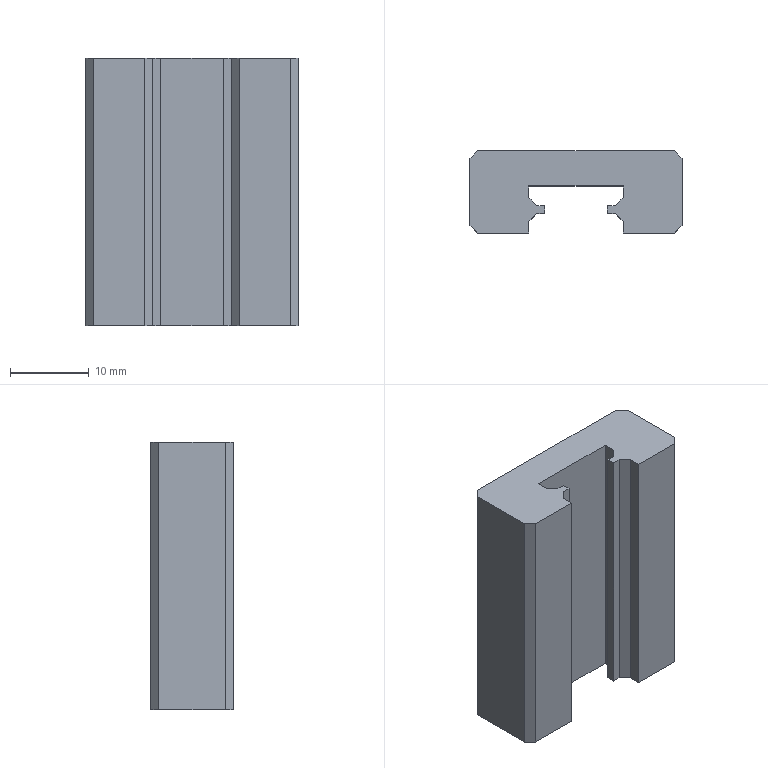Part | SolidWorks | features Chamfer 1, Extrusion 1 | 1 solid | 26 faces | box 27 x 10.5 x 34 mm | volume 7327 mm3 | plane 26
STEP:
#1=CARTESIAN_POINT('',(6.,-5.5,0.));
#2=VERTEX_POINT('',#1);
#3=CARTESIAN_POINT('',(12.5,-5.5,0.));
#4=VERTEX_POINT('',#3);
#5=CARTESIAN_POINT('',(6.,-5.5,0.));
#6=DIRECTION('',(1.,0.,0.));
#7=VECTOR('',#6,1000.);
#8=LINE('',#5,#7);
#9=EDGE_CURVE('',#2,#4,#8,.T.);
#10=ORIENTED_EDGE('',*,*,#9,.T.);
#11=CARTESIAN_POINT('',(12.5,-5.5,34.));
#12=VERTEX_POINT('',#11);
#13=CARTESIAN_POINT('',(12.5,-5.5,34.));
#14=DIRECTION('',(0.,0.,1.));
#15=VECTOR('',#14,1000.);
#16=LINE('',#13,#15);
#17=EDGE_CURVE('',#4,#12,#16,.T.);
#18=ORIENTED_EDGE('',*,*,#17,.T.);
#19=CARTESIAN_POINT('',(6.,-5.5,34.));
#20=VERTEX_POINT('',#19);
#21=CARTESIAN_POINT('',(6.,-5.5,34.));
#22=DIRECTION('',(1.,0.,0.));
#23=VECTOR('',#22,1000.);
#24=LINE('',#21,#23);
#25=EDGE_CURVE('',#20,#12,#24,.T.);
#26=ORIENTED_EDGE('',*,*,#25,.F.);
#27=CARTESIAN_POINT('',(6.,-5.5,34.));
#28=DIRECTION('',(0.,0.,-1.));
#29=VECTOR('',#28,1000.);
#30=LINE('',#27,#29);
#31=EDGE_CURVE('',#20,#2,#30,.T.);
#32=ORIENTED_EDGE('',*,*,#31,.T.);
#33=EDGE_LOOP('',(#10,#18,#26,#32));
#34=FACE_OUTER_BOUND('',#33,.T.);
#35=CARTESIAN_POINT('',(6.,-5.5,34.));
#36=DIRECTION('',(0.,1.,0.));
#37=DIRECTION('',(0.,0.,1.));
#38=AXIS2_PLACEMENT_3D('',#35,#36,#37);
#39=PLANE('',#38);
#40=ADVANCED_FACE('',(#34),#39,.F.);
#41=CARTESIAN_POINT('',(13.5,-4.5,34.));
#42=VERTEX_POINT('',#41);
#43=CARTESIAN_POINT('',(13.5,4.,34.));
#44=VERTEX_POINT('',#43);
#45=CARTESIAN_POINT('',(13.5,5.,34.));
#46=DIRECTION('',(0.,1.,0.));
#47=VECTOR('',#46,1000.);
#48=LINE('',#45,#47);
#49=EDGE_CURVE('',#42,#44,#48,.T.);
#50=ORIENTED_EDGE('',*,*,#49,.F.);
#51=CARTESIAN_POINT('',(13.5,-4.5,0.));
#52=VERTEX_POINT('',#51);
#53=CARTESIAN_POINT('',(13.5,-4.5,34.));
#54=DIRECTION('',(0.,0.,-1.));
#55=VECTOR('',#54,1000.);
#56=LINE('',#53,#55);
#57=EDGE_CURVE('',#42,#52,#56,.T.);
#58=ORIENTED_EDGE('',*,*,#57,.T.);
#59=CARTESIAN_POINT('',(13.5,4.,0.));
#60=VERTEX_POINT('',#59);
#61=CARTESIAN_POINT('',(13.5,5.,0.));
#62=DIRECTION('',(0.,1.,0.));
#63=VECTOR('',#62,1000.);
#64=LINE('',#61,#63);
#65=EDGE_CURVE('',#52,#60,#64,.T.);
#66=ORIENTED_EDGE('',*,*,#65,.T.);
#67=CARTESIAN_POINT('',(13.5,4.,34.));
#68=DIRECTION('',(0.,0.,1.));
#69=VECTOR('',#68,1000.);
#70=LINE('',#67,#69);
#71=EDGE_CURVE('',#60,#44,#70,.T.);
#72=ORIENTED_EDGE('',*,*,#71,.T.);
#73=EDGE_LOOP('',(#50,#58,#66,#72));
#74=FACE_OUTER_BOUND('',#73,.T.);
#75=CARTESIAN_POINT('',(13.5,5.,34.));
#76=DIRECTION('',(-1.,0.,0.));
#77=DIRECTION('',(0.,-1.,0.));
#78=AXIS2_PLACEMENT_3D('',#75,#76,#77);
#79=PLANE('',#78);
#80=ADVANCED_FACE('',(#74),#79,.F.);
#81=CARTESIAN_POINT('',(12.5,5.,0.));
#82=VERTEX_POINT('',#81);
#83=CARTESIAN_POINT('',(-12.5,5.,0.));
#84=VERTEX_POINT('',#83);
#85=CARTESIAN_POINT('',(-13.5,5.,0.));
#86=DIRECTION('',(-1.,0.,0.));
#87=VECTOR('',#86,1000.);
#88=LINE('',#85,#87);
#89=EDGE_CURVE('',#82,#84,#88,.T.);
#90=ORIENTED_EDGE('',*,*,#89,.T.);
#91=CARTESIAN_POINT('',(-12.5,5.,34.));
#92=VERTEX_POINT('',#91);
#93=CARTESIAN_POINT('',(-12.5,5.,34.));
#94=DIRECTION('',(0.,0.,1.));
#95=VECTOR('',#94,1000.);
#96=LINE('',#93,#95);
#97=EDGE_CURVE('',#84,#92,#96,.T.);
#98=ORIENTED_EDGE('',*,*,#97,.T.);
#99=CARTESIAN_POINT('',(12.5,5.,34.));
#100=VERTEX_POINT('',#99);
#101=CARTESIAN_POINT('',(-13.5,5.,34.));
#102=DIRECTION('',(-1.,0.,0.));
#103=VECTOR('',#102,1000.);
#104=LINE('',#101,#103);
#105=EDGE_CURVE('',#100,#92,#104,.T.);
#106=ORIENTED_EDGE('',*,*,#105,.F.);
#107=CARTESIAN_POINT('',(12.5,5.,34.));
#108=DIRECTION('',(0.,0.,-1.));
#109=VECTOR('',#108,1000.);
#110=LINE('',#107,#109);
#111=EDGE_CURVE('',#100,#82,#110,.T.);
#112=ORIENTED_EDGE('',*,*,#111,.T.);
#113=EDGE_LOOP('',(#90,#98,#106,#112));
#114=FACE_OUTER_BOUND('',#113,.T.);
#115=CARTESIAN_POINT('',(-13.5,5.,34.));
#116=DIRECTION('',(0.,-1.,0.));
#117=DIRECTION('',(0.,0.,-1.));
#118=AXIS2_PLACEMENT_3D('',#115,#116,#117);
#119=PLANE('',#118);
#120=ADVANCED_FACE('',(#114),#119,.F.);
#121=CARTESIAN_POINT('',(-13.5,4.,0.));
#122=VERTEX_POINT('',#121);
#123=CARTESIAN_POINT('',(-13.5,-4.5,0.));
#124=VERTEX_POINT('',#123);
#125=CARTESIAN_POINT('',(-13.5,5.,0.));
#126=DIRECTION('',(0.,-1.,0.));
#127=VECTOR('',#126,1000.);
#128=LINE('',#125,#127);
#129=EDGE_CURVE('',#122,#124,#128,.T.);
#130=ORIENTED_EDGE('',*,*,#129,.T.);
#131=CARTESIAN_POINT('',(-13.5,-4.5,34.));
#132=VERTEX_POINT('',#131);
#133=CARTESIAN_POINT('',(-13.5,-4.5,34.));
#134=DIRECTION('',(0.,0.,1.));
#135=VECTOR('',#134,1000.);
#136=LINE('',#133,#135);
#137=EDGE_CURVE('',#124,#132,#136,.T.);
#138=ORIENTED_EDGE('',*,*,#137,.T.);
#139=CARTESIAN_POINT('',(-13.5,4.,34.));
#140=VERTEX_POINT('',#139);
#141=CARTESIAN_POINT('',(-13.5,5.,34.));
#142=DIRECTION('',(0.,-1.,0.));
#143=VECTOR('',#142,1000.);
#144=LINE('',#141,#143);
#145=EDGE_CURVE('',#140,#132,#144,.T.);
#146=ORIENTED_EDGE('',*,*,#145,.F.);
#147=CARTESIAN_POINT('',(-13.5,4.,34.));
#148=DIRECTION('',(0.,0.,-1.));
#149=VECTOR('',#148,1000.);
#150=LINE('',#147,#149);
#151=EDGE_CURVE('',#140,#122,#150,.T.);
#152=ORIENTED_EDGE('',*,*,#151,.T.);
#153=EDGE_LOOP('',(#130,#138,#146,#152));
#154=FACE_OUTER_BOUND('',#153,.T.);
#155=CARTESIAN_POINT('',(-13.5,5.,34.));
#156=DIRECTION('',(1.,0.,0.));
#157=DIRECTION('',(0.,1.,0.));
#158=AXIS2_PLACEMENT_3D('',#155,#156,#157);
#159=PLANE('',#158);
#160=ADVANCED_FACE('',(#154),#159,.F.);
#161=CARTESIAN_POINT('',(-12.5,-5.5,34.));
#162=VERTEX_POINT('',#161);
#163=CARTESIAN_POINT('',(-6.,-5.5,34.));
#164=VERTEX_POINT('',#163);
#165=CARTESIAN_POINT('',(-13.5,-5.5,34.));
#166=DIRECTION('',(1.,0.,0.));
#167=VECTOR('',#166,1000.);
#168=LINE('',#165,#167);
#169=EDGE_CURVE('',#162,#164,#168,.T.);
#170=ORIENTED_EDGE('',*,*,#169,.F.);
#171=CARTESIAN_POINT('',(-12.5,-5.5,0.));
#172=VERTEX_POINT('',#171);
#173=CARTESIAN_POINT('',(-12.5,-5.5,34.));
#174=DIRECTION('',(0.,0.,-1.));
#175=VECTOR('',#174,1000.);
#176=LINE('',#173,#175);
#177=EDGE_CURVE('',#162,#172,#176,.T.);
#178=ORIENTED_EDGE('',*,*,#177,.T.);
#179=CARTESIAN_POINT('',(-6.,-5.5,0.));
#180=VERTEX_POINT('',#179);
#181=CARTESIAN_POINT('',(-13.5,-5.5,0.));
#182=DIRECTION('',(1.,0.,0.));
#183=VECTOR('',#182,1000.);
#184=LINE('',#181,#183);
#185=EDGE_CURVE('',#172,#180,#184,.T.);
#186=ORIENTED_EDGE('',*,*,#185,.T.);
#187=CARTESIAN_POINT('',(-6.,-5.5,34.));
#188=DIRECTION('',(0.,0.,-1.));
#189=VECTOR('',#188,1000.);
#190=LINE('',#187,#189);
#191=EDGE_CURVE('',#164,#180,#190,.T.);
#192=ORIENTED_EDGE('',*,*,#191,.F.);
#193=EDGE_LOOP('',(#170,#178,#186,#192));
#194=FACE_OUTER_BOUND('',#193,.T.);
#195=CARTESIAN_POINT('',(-13.5,-5.5,34.));
#196=DIRECTION('',(0.,1.,0.));
#197=DIRECTION('',(0.,0.,1.));
#198=AXIS2_PLACEMENT_3D('',#195,#196,#197);
#199=PLANE('',#198);
#200=ADVANCED_FACE('',(#194),#199,.F.);
#201=CARTESIAN_POINT('',(-6.,-4.,0.));
#202=VERTEX_POINT('',#201);
#203=CARTESIAN_POINT('',(-6.,-4.,0.));
#204=DIRECTION('',(0.,1.,0.));
#205=VECTOR('',#204,1000.);
#206=LINE('',#203,#205);
#207=EDGE_CURVE('',#180,#202,#206,.T.);
#208=ORIENTED_EDGE('',*,*,#207,.T.);
#209=CARTESIAN_POINT('',(-6.,-4.,34.));
#210=VERTEX_POINT('',#209);
#211=CARTESIAN_POINT('',(-6.,-4.,34.));
#212=DIRECTION('',(0.,0.,-1.));
#213=VECTOR('',#212,1000.);
#214=LINE('',#211,#213);
#215=EDGE_CURVE('',#210,#202,#214,.T.);
#216=ORIENTED_EDGE('',*,*,#215,.F.);
#217=CARTESIAN_POINT('',(-6.,-4.,34.));
#218=DIRECTION('',(0.,1.,0.));
#219=VECTOR('',#218,1000.);
#220=LINE('',#217,#219);
#221=EDGE_CURVE('',#164,#210,#220,.T.);
#222=ORIENTED_EDGE('',*,*,#221,.F.);
#223=ORIENTED_EDGE('',*,*,#191,.T.);
#224=EDGE_LOOP('',(#208,#216,#222,#223));
#225=FACE_OUTER_BOUND('',#224,.T.);
#226=CARTESIAN_POINT('',(-6.,-4.,34.));
#227=DIRECTION('',(-1.,0.,0.));
#228=DIRECTION('',(0.,-1.,0.));
#229=AXIS2_PLACEMENT_3D('',#226,#227,#228);
#230=PLANE('',#229);
#231=ADVANCED_FACE('',(#225),#230,.F.);
#232=CARTESIAN_POINT('',(-5.,-3.,0.));
#233=VERTEX_POINT('',#232);
#234=CARTESIAN_POINT('',(-5.,-3.,0.));
#235=DIRECTION('',(0.7071,0.7071,0.));
#236=VECTOR('',#235,1000.);
#237=LINE('',#234,#236);
#238=EDGE_CURVE('',#202,#233,#237,.T.);
#239=ORIENTED_EDGE('',*,*,#238,.T.);
#240=CARTESIAN_POINT('',(-5.,-3.,34.));
#241=VERTEX_POINT('',#240);
#242=CARTESIAN_POINT('',(-5.,-3.,34.));
#243=DIRECTION('',(0.,0.,-1.));
#244=VECTOR('',#243,1000.);
#245=LINE('',#242,#244);
#246=EDGE_CURVE('',#241,#233,#245,.T.);
#247=ORIENTED_EDGE('',*,*,#246,.F.);
#248=CARTESIAN_POINT('',(-5.,-3.,34.));
#249=DIRECTION('',(0.7071,0.7071,0.));
#250=VECTOR('',#249,1000.);
#251=LINE('',#248,#250);
#252=EDGE_CURVE('',#210,#241,#251,.T.);
#253=ORIENTED_EDGE('',*,*,#252,.F.);
#254=ORIENTED_EDGE('',*,*,#215,.T.);
#255=EDGE_LOOP('',(#239,#247,#253,#254));
#256=FACE_OUTER_BOUND('',#255,.T.);
#257=CARTESIAN_POINT('',(-5.,-3.,34.));
#258=DIRECTION('',(-0.7071,0.7071,0.));
#259=DIRECTION('',(-0.7071,-0.7071,0.));
#260=AXIS2_PLACEMENT_3D('',#257,#258,#259);
#261=PLANE('',#260);
#262=ADVANCED_FACE('',(#256),#261,.F.);
#263=CARTESIAN_POINT('',(-4.,-3.,0.));
#264=VERTEX_POINT('',#263);
#265=CARTESIAN_POINT('',(-4.,-3.,0.));
#266=DIRECTION('',(1.,0.,0.));
#267=VECTOR('',#266,1000.);
#268=LINE('',#265,#267);
#269=EDGE_CURVE('',#233,#264,#268,.T.);
#270=ORIENTED_EDGE('',*,*,#269,.T.);
#271=CARTESIAN_POINT('',(-4.,-3.,34.));
#272=VERTEX_POINT('',#271);
#273=CARTESIAN_POINT('',(-4.,-3.,34.));
#274=DIRECTION('',(0.,0.,-1.));
#275=VECTOR('',#274,1000.);
#276=LINE('',#273,#275);
#277=EDGE_CURVE('',#272,#264,#276,.T.);
#278=ORIENTED_EDGE('',*,*,#277,.F.);
#279=CARTESIAN_POINT('',(-4.,-3.,34.));
#280=DIRECTION('',(1.,0.,0.));
#281=VECTOR('',#280,1000.);
#282=LINE('',#279,#281);
#283=EDGE_CURVE('',#241,#272,#282,.T.);
#284=ORIENTED_EDGE('',*,*,#283,.F.);
#285=ORIENTED_EDGE('',*,*,#246,.T.);
#286=EDGE_LOOP('',(#270,#278,#284,#285));
#287=FACE_OUTER_BOUND('',#286,.T.);
#288=CARTESIAN_POINT('',(-4.,-3.,34.));
#289=DIRECTION('',(0.,1.,0.));
#290=DIRECTION('',(0.,0.,1.));
#291=AXIS2_PLACEMENT_3D('',#288,#289,#290);
#292=PLANE('',#291);
#293=ADVANCED_FACE('',(#287),#292,.F.);
#294=CARTESIAN_POINT('',(-4.,-2.,0.));
#295=VERTEX_POINT('',#294);
#296=CARTESIAN_POINT('',(-4.,-2.,0.));
#297=DIRECTION('',(0.,1.,0.));
#298=VECTOR('',#297,1000.);
#299=LINE('',#296,#298);
#300=EDGE_CURVE('',#264,#295,#299,.T.);
#301=ORIENTED_EDGE('',*,*,#300,.T.);
#302=CARTESIAN_POINT('',(-4.,-2.,34.));
#303=VERTEX_POINT('',#302);
#304=CARTESIAN_POINT('',(-4.,-2.,34.));
#305=DIRECTION('',(0.,0.,-1.));
#306=VECTOR('',#305,1000.);
#307=LINE('',#304,#306);
#308=EDGE_CURVE('',#303,#295,#307,.T.);
#309=ORIENTED_EDGE('',*,*,#308,.F.);
#310=CARTESIAN_POINT('',(-4.,-2.,34.));
#311=DIRECTION('',(0.,1.,0.));
#312=VECTOR('',#311,1000.);
#313=LINE('',#310,#312);
#314=EDGE_CURVE('',#272,#303,#313,.T.);
#315=ORIENTED_EDGE('',*,*,#314,.F.);
#316=ORIENTED_EDGE('',*,*,#277,.T.);
#317=EDGE_LOOP('',(#301,#309,#315,#316));
#318=FACE_OUTER_BOUND('',#317,.T.);
#319=CARTESIAN_POINT('',(-4.,-2.,34.));
#320=DIRECTION('',(-1.,0.,0.));
#321=DIRECTION('',(0.,-1.,0.));
#322=AXIS2_PLACEMENT_3D('',#319,#320,#321);
#323=PLANE('',#322);
#324=ADVANCED_FACE('',(#318),#323,.F.);
#325=CARTESIAN_POINT('',(-5.,-2.,0.));
#326=VERTEX_POINT('',#325);
#327=CARTESIAN_POINT('',(-4.,-2.,0.));
#328=DIRECTION('',(-1.,0.,0.));
#329=VECTOR('',#328,1000.);
#330=LINE('',#327,#329);
#331=EDGE_CURVE('',#295,#326,#330,.T.);
#332=ORIENTED_EDGE('',*,*,#331,.T.);
#333=CARTESIAN_POINT('',(-5.,-2.,34.));
#334=VERTEX_POINT('',#333);
#335=CARTESIAN_POINT('',(-5.,-2.,34.));
#336=DIRECTION('',(0.,0.,-1.));
#337=VECTOR('',#336,1000.);
#338=LINE('',#335,#337);
#339=EDGE_CURVE('',#334,#326,#338,.T.);
#340=ORIENTED_EDGE('',*,*,#339,.F.);
#341=CARTESIAN_POINT('',(-4.,-2.,34.));
#342=DIRECTION('',(-1.,0.,0.));
#343=VECTOR('',#342,1000.);
#344=LINE('',#341,#343);
#345=EDGE_CURVE('',#303,#334,#344,.T.);
#346=ORIENTED_EDGE('',*,*,#345,.F.);
#347=ORIENTED_EDGE('',*,*,#308,.T.);
#348=EDGE_LOOP('',(#332,#340,#346,#347));
#349=FACE_OUTER_BOUND('',#348,.T.);
#350=CARTESIAN_POINT('',(-4.,-2.,34.));
#351=DIRECTION('',(0.,-1.,0.));
#352=DIRECTION('',(0.,0.,-1.));
#353=AXIS2_PLACEMENT_3D('',#350,#351,#352);
#354=PLANE('',#353);
#355=ADVANCED_FACE('',(#349),#354,.F.);
#356=CARTESIAN_POINT('',(-6.,-1.,0.));
#357=VERTEX_POINT('',#356);
#358=CARTESIAN_POINT('',(-5.,-2.,0.));
#359=DIRECTION('',(-0.7071,0.7071,0.));
#360=VECTOR('',#359,1000.);
#361=LINE('',#358,#360);
#362=EDGE_CURVE('',#326,#357,#361,.T.);
#363=ORIENTED_EDGE('',*,*,#362,.T.);
#364=CARTESIAN_POINT('',(-6.,-1.,34.));
#365=VERTEX_POINT('',#364);
#366=CARTESIAN_POINT('',(-6.,-1.,34.));
#367=DIRECTION('',(0.,0.,-1.));
#368=VECTOR('',#367,1000.);
#369=LINE('',#366,#368);
#370=EDGE_CURVE('',#365,#357,#369,.T.);
#371=ORIENTED_EDGE('',*,*,#370,.F.);
#372=CARTESIAN_POINT('',(-5.,-2.,34.));
#373=DIRECTION('',(-0.7071,0.7071,0.));
#374=VECTOR('',#373,1000.);
#375=LINE('',#372,#374);
#376=EDGE_CURVE('',#334,#365,#375,.T.);
#377=ORIENTED_EDGE('',*,*,#376,.F.);
#378=ORIENTED_EDGE('',*,*,#339,.T.);
#379=EDGE_LOOP('',(#363,#371,#377,#378));
#380=FACE_OUTER_BOUND('',#379,.T.);
#381=CARTESIAN_POINT('',(-5.,-2.,34.));
#382=DIRECTION('',(-0.7071,-0.7071,0.));
#383=DIRECTION('',(0.7071,-0.7071,0.));
#384=AXIS2_PLACEMENT_3D('',#381,#382,#383);
#385=PLANE('',#384);
#386=ADVANCED_FACE('',(#380),#385,.F.);
#387=CARTESIAN_POINT('',(-6.,0.5,0.));
#388=VERTEX_POINT('',#387);
#389=CARTESIAN_POINT('',(-6.,0.5,0.));
#390=DIRECTION('',(0.,1.,0.));
#391=VECTOR('',#390,1000.);
#392=LINE('',#389,#391);
#393=EDGE_CURVE('',#357,#388,#392,.T.);
#394=ORIENTED_EDGE('',*,*,#393,.T.);
#395=CARTESIAN_POINT('',(-6.,0.5,34.));
#396=VERTEX_POINT('',#395);
#397=CARTESIAN_POINT('',(-6.,0.5,34.));
#398=DIRECTION('',(0.,0.,-1.));
#399=VECTOR('',#398,1000.);
#400=LINE('',#397,#399);
#401=EDGE_CURVE('',#396,#388,#400,.T.);
#402=ORIENTED_EDGE('',*,*,#401,.F.);
#403=CARTESIAN_POINT('',(-6.,0.5,34.));
#404=DIRECTION('',(0.,1.,0.));
#405=VECTOR('',#404,1000.);
#406=LINE('',#403,#405);
#407=EDGE_CURVE('',#365,#396,#406,.T.);
#408=ORIENTED_EDGE('',*,*,#407,.F.);
#409=ORIENTED_EDGE('',*,*,#370,.T.);
#410=EDGE_LOOP('',(#394,#402,#408,#409));
#411=FACE_OUTER_BOUND('',#410,.T.);
#412=CARTESIAN_POINT('',(-6.,0.5,34.));
#413=DIRECTION('',(-1.,0.,0.));
#414=DIRECTION('',(0.,0.,1.));
#415=AXIS2_PLACEMENT_3D('',#412,#413,#414);
#416=PLANE('',#415);
#417=ADVANCED_FACE('',(#411),#416,.F.);
#418=CARTESIAN_POINT('',(6.,0.5,0.));
#419=VERTEX_POINT('',#418);
#420=CARTESIAN_POINT('',(-6.,0.5,0.));
#421=DIRECTION('',(1.,0.,0.));
#422=VECTOR('',#421,1000.);
#423=LINE('',#420,#422);
#424=EDGE_CURVE('',#388,#419,#423,.T.);
#425=ORIENTED_EDGE('',*,*,#424,.T.);
#426=CARTESIAN_POINT('',(6.,0.5,34.));
#427=VERTEX_POINT('',#426);
#428=CARTESIAN_POINT('',(6.,0.5,34.));
#429=DIRECTION('',(0.,0.,-1.));
#430=VECTOR('',#429,1000.);
#431=LINE('',#428,#430);
#432=EDGE_CURVE('',#427,#419,#431,.T.);
#433=ORIENTED_EDGE('',*,*,#432,.F.);
#434=CARTESIAN_POINT('',(-6.,0.5,34.));
#435=DIRECTION('',(1.,0.,0.));
#436=VECTOR('',#435,1000.);
#437=LINE('',#434,#436);
#438=EDGE_CURVE('',#396,#427,#437,.T.);
#439=ORIENTED_EDGE('',*,*,#438,.F.);
#440=ORIENTED_EDGE('',*,*,#401,.T.);
#441=EDGE_LOOP('',(#425,#433,#439,#440));
#442=FACE_OUTER_BOUND('',#441,.T.);
#443=CARTESIAN_POINT('',(-6.,0.5,34.));
#444=DIRECTION('',(0.,1.,0.));
#445=DIRECTION('',(0.,0.,1.));
#446=AXIS2_PLACEMENT_3D('',#443,#444,#445);
#447=PLANE('',#446);
#448=ADVANCED_FACE('',(#442),#447,.F.);
#449=CARTESIAN_POINT('',(6.,-1.,0.));
#450=VERTEX_POINT('',#449);
#451=CARTESIAN_POINT('',(6.,0.5,0.));
#452=DIRECTION('',(0.,-1.,0.));
#453=VECTOR('',#452,1000.);
#454=LINE('',#451,#453);
#455=EDGE_CURVE('',#419,#450,#454,.T.);
#456=ORIENTED_EDGE('',*,*,#455,.T.);
#457=CARTESIAN_POINT('',(6.,-1.,34.));
#458=VERTEX_POINT('',#457);
#459=CARTESIAN_POINT('',(6.,-1.,34.));
#460=DIRECTION('',(0.,0.,-1.));
#461=VECTOR('',#460,1000.);
#462=LINE('',#459,#461);
#463=EDGE_CURVE('',#458,#450,#462,.T.);
#464=ORIENTED_EDGE('',*,*,#463,.F.);
#465=CARTESIAN_POINT('',(6.,0.5,34.));
#466=DIRECTION('',(0.,-1.,0.));
#467=VECTOR('',#466,1000.);
#468=LINE('',#465,#467);
#469=EDGE_CURVE('',#427,#458,#468,.T.);
#470=ORIENTED_EDGE('',*,*,#469,.F.);
#471=ORIENTED_EDGE('',*,*,#432,.T.);
#472=EDGE_LOOP('',(#456,#464,#470,#471));
#473=FACE_OUTER_BOUND('',#472,.T.);
#474=CARTESIAN_POINT('',(6.,0.5,34.));
#475=DIRECTION('',(1.,0.,0.));
#476=DIRECTION('',(0.,0.,-1.));
#477=AXIS2_PLACEMENT_3D('',#474,#475,#476);
#478=PLANE('',#477);
#479=ADVANCED_FACE('',(#473),#478,.F.);
#480=CARTESIAN_POINT('',(5.,-2.,0.));
#481=VERTEX_POINT('',#480);
#482=CARTESIAN_POINT('',(5.,-2.,0.));
#483=DIRECTION('',(-0.7071,-0.7071,0.));
#484=VECTOR('',#483,1000.);
#485=LINE('',#482,#484);
#486=EDGE_CURVE('',#450,#481,#485,.T.);
#487=ORIENTED_EDGE('',*,*,#486,.T.);
#488=CARTESIAN_POINT('',(5.,-2.,34.));
#489=VERTEX_POINT('',#488);
#490=CARTESIAN_POINT('',(5.,-2.,34.));
#491=DIRECTION('',(0.,0.,-1.));
#492=VECTOR('',#491,1000.);
#493=LINE('',#490,#492);
#494=EDGE_CURVE('',#489,#481,#493,.T.);
#495=ORIENTED_EDGE('',*,*,#494,.F.);
#496=CARTESIAN_POINT('',(5.,-2.,34.));
#497=DIRECTION('',(-0.7071,-0.7071,0.));
#498=VECTOR('',#497,1000.);
#499=LINE('',#496,#498);
#500=EDGE_CURVE('',#458,#489,#499,.T.);
#501=ORIENTED_EDGE('',*,*,#500,.F.);
#502=ORIENTED_EDGE('',*,*,#463,.T.);
#503=EDGE_LOOP('',(#487,#495,#501,#502));
#504=FACE_OUTER_BOUND('',#503,.T.);
#505=CARTESIAN_POINT('',(5.,-2.,34.));
#506=DIRECTION('',(0.7071,-0.7071,0.));
#507=DIRECTION('',(0.7071,0.7071,0.));
#508=AXIS2_PLACEMENT_3D('',#505,#506,#507);
#509=PLANE('',#508);
#510=ADVANCED_FACE('',(#504),#509,.F.);
#511=CARTESIAN_POINT('',(4.,-2.,0.));
#512=VERTEX_POINT('',#511);
#513=CARTESIAN_POINT('',(4.,-2.,0.));
#514=DIRECTION('',(-1.,0.,0.));
#515=VECTOR('',#514,1000.);
#516=LINE('',#513,#515);
#517=EDGE_CURVE('',#481,#512,#516,.T.);
#518=ORIENTED_EDGE('',*,*,#517,.T.);
#519=CARTESIAN_POINT('',(4.,-2.,34.));
#520=VERTEX_POINT('',#519);
#521=CARTESIAN_POINT('',(4.,-2.,34.));
#522=DIRECTION('',(0.,0.,-1.));
#523=VECTOR('',#522,1000.);
#524=LINE('',#521,#523);
#525=EDGE_CURVE('',#520,#512,#524,.T.);
#526=ORIENTED_EDGE('',*,*,#525,.F.);
#527=CARTESIAN_POINT('',(4.,-2.,34.));
#528=DIRECTION('',(-1.,0.,0.));
#529=VECTOR('',#528,1000.);
#530=LINE('',#527,#529);
#531=EDGE_CURVE('',#489,#520,#530,.T.);
#532=ORIENTED_EDGE('',*,*,#531,.F.);
#533=ORIENTED_EDGE('',*,*,#494,.T.);
#534=EDGE_LOOP('',(#518,#526,#532,#533));
#535=FACE_OUTER_BOUND('',#534,.T.);
#536=CARTESIAN_POINT('',(4.,-2.,34.));
#537=DIRECTION('',(0.,-1.,0.));
#538=DIRECTION('',(0.,0.,-1.));
#539=AXIS2_PLACEMENT_3D('',#536,#537,#538);
#540=PLANE('',#539);
#541=ADVANCED_FACE('',(#535),#540,.F.);
#542=CARTESIAN_POINT('',(4.,-3.,0.));
#543=VERTEX_POINT('',#542);
#544=CARTESIAN_POINT('',(4.,-2.,0.));
#545=DIRECTION('',(0.,-1.,0.));
#546=VECTOR('',#545,1000.);
#547=LINE('',#544,#546);
#548=EDGE_CURVE('',#512,#543,#547,.T.);
#549=ORIENTED_EDGE('',*,*,#548,.T.);
#550=CARTESIAN_POINT('',(4.,-3.,34.));
#551=VERTEX_POINT('',#550);
#552=CARTESIAN_POINT('',(4.,-3.,34.));
#553=DIRECTION('',(0.,0.,-1.));
#554=VECTOR('',#553,1000.);
#555=LINE('',#552,#554);
#556=EDGE_CURVE('',#551,#543,#555,.T.);
#557=ORIENTED_EDGE('',*,*,#556,.F.);
#558=CARTESIAN_POINT('',(4.,-2.,34.));
#559=DIRECTION('',(0.,-1.,0.));
#560=VECTOR('',#559,1000.);
#561=LINE('',#558,#560);
#562=EDGE_CURVE('',#520,#551,#561,.T.);
#563=ORIENTED_EDGE('',*,*,#562,.F.);
#564=ORIENTED_EDGE('',*,*,#525,.T.);
#565=EDGE_LOOP('',(#549,#557,#563,#564));
#566=FACE_OUTER_BOUND('',#565,.T.);
#567=CARTESIAN_POINT('',(4.,-2.,34.));
#568=DIRECTION('',(1.,0.,0.));
#569=DIRECTION('',(0.,0.,-1.));
#570=AXIS2_PLACEMENT_3D('',#567,#568,#569);
#571=PLANE('',#570);
#572=ADVANCED_FACE('',(#566),#571,.F.);
#573=CARTESIAN_POINT('',(5.,-3.,0.));
#574=VERTEX_POINT('',#573);
#575=CARTESIAN_POINT('',(4.,-3.,0.));
#576=DIRECTION('',(1.,0.,0.));
#577=VECTOR('',#576,1000.);
#578=LINE('',#575,#577);
#579=EDGE_CURVE('',#543,#574,#578,.T.);
#580=ORIENTED_EDGE('',*,*,#579,.T.);
#581=CARTESIAN_POINT('',(5.,-3.,34.));
#582=VERTEX_POINT('',#581);
#583=CARTESIAN_POINT('',(5.,-3.,34.));
#584=DIRECTION('',(0.,0.,-1.));
#585=VECTOR('',#584,1000.);
#586=LINE('',#583,#585);
#587=EDGE_CURVE('',#582,#574,#586,.T.);
#588=ORIENTED_EDGE('',*,*,#587,.F.);
#589=CARTESIAN_POINT('',(4.,-3.,34.));
#590=DIRECTION('',(1.,0.,0.));
#591=VECTOR('',#590,1000.);
#592=LINE('',#589,#591);
#593=EDGE_CURVE('',#551,#582,#592,.T.);
#594=ORIENTED_EDGE('',*,*,#593,.F.);
#595=ORIENTED_EDGE('',*,*,#556,.T.);
#596=EDGE_LOOP('',(#580,#588,#594,#595));
#597=FACE_OUTER_BOUND('',#596,.T.);
#598=CARTESIAN_POINT('',(4.,-3.,34.));
#599=DIRECTION('',(0.,1.,0.));
#600=DIRECTION('',(-1.,0.,0.));
#601=AXIS2_PLACEMENT_3D('',#598,#599,#600);
#602=PLANE('',#601);
#603=ADVANCED_FACE('',(#597),#602,.F.);
#604=CARTESIAN_POINT('',(6.,-4.,0.));
#605=VERTEX_POINT('',#604);
#606=CARTESIAN_POINT('',(5.,-3.,0.));
#607=DIRECTION('',(0.7071,-0.7071,0.));
#608=VECTOR('',#607,1000.);
#609=LINE('',#606,#608);
#610=EDGE_CURVE('',#574,#605,#609,.T.);
#611=ORIENTED_EDGE('',*,*,#610,.T.);
#612=CARTESIAN_POINT('',(6.,-4.,34.));
#613=VERTEX_POINT('',#612);
#614=CARTESIAN_POINT('',(6.,-4.,34.));
#615=DIRECTION('',(0.,0.,-1.));
#616=VECTOR('',#615,1000.);
#617=LINE('',#614,#616);
#618=EDGE_CURVE('',#613,#605,#617,.T.);
#619=ORIENTED_EDGE('',*,*,#618,.F.);
#620=CARTESIAN_POINT('',(5.,-3.,34.));
#621=DIRECTION('',(0.7071,-0.7071,0.));
#622=VECTOR('',#621,1000.);
#623=LINE('',#620,#622);
#624=EDGE_CURVE('',#582,#613,#623,.T.);
#625=ORIENTED_EDGE('',*,*,#624,.F.);
#626=ORIENTED_EDGE('',*,*,#587,.T.);
#627=EDGE_LOOP('',(#611,#619,#625,#626));
#628=FACE_OUTER_BOUND('',#627,.T.);
#629=CARTESIAN_POINT('',(5.,-3.,34.));
#630=DIRECTION('',(0.7071,0.7071,0.));
#631=DIRECTION('',(-0.7071,0.7071,0.));
#632=AXIS2_PLACEMENT_3D('',#629,#630,#631);
#633=PLANE('',#632);
#634=ADVANCED_FACE('',(#628),#633,.F.);
#635=CARTESIAN_POINT('',(6.,-4.,0.));
#636=DIRECTION('',(0.,-1.,0.));
#637=VECTOR('',#636,1000.);
#638=LINE('',#635,#637);
#639=EDGE_CURVE('',#605,#2,#638,.T.);
#640=ORIENTED_EDGE('',*,*,#639,.T.);
#641=ORIENTED_EDGE('',*,*,#31,.F.);
#642=CARTESIAN_POINT('',(6.,-4.,34.));
#643=DIRECTION('',(0.,-1.,0.));
#644=VECTOR('',#643,1000.);
#645=LINE('',#642,#644);
#646=EDGE_CURVE('',#613,#20,#645,.T.);
#647=ORIENTED_EDGE('',*,*,#646,.F.);
#648=ORIENTED_EDGE('',*,*,#618,.T.);
#649=EDGE_LOOP('',(#640,#641,#647,#648));
#650=FACE_OUTER_BOUND('',#649,.T.);
#651=CARTESIAN_POINT('',(6.,-4.,34.));
#652=DIRECTION('',(1.,0.,0.));
#653=DIRECTION('',(0.,1.,0.));
#654=AXIS2_PLACEMENT_3D('',#651,#652,#653);
#655=PLANE('',#654);
#656=ADVANCED_FACE('',(#650),#655,.F.);
#657=ORIENTED_EDGE('',*,*,#25,.T.);
#658=CARTESIAN_POINT('',(13.5,-4.5,34.));
#659=DIRECTION('',(0.7071,0.7071,0.));
#660=VECTOR('',#659,1000.);
#661=LINE('',#658,#660);
#662=EDGE_CURVE('',#12,#42,#661,.T.);
#663=ORIENTED_EDGE('',*,*,#662,.T.);
#664=ORIENTED_EDGE('',*,*,#49,.T.);
#665=CARTESIAN_POINT('',(12.5,5.,34.));
#666=DIRECTION('',(-0.7071,0.7071,0.));
#667=VECTOR('',#666,1000.);
#668=LINE('',#665,#667);
#669=EDGE_CURVE('',#44,#100,#668,.T.);
#670=ORIENTED_EDGE('',*,*,#669,.T.);
#671=ORIENTED_EDGE('',*,*,#105,.T.);
#672=CARTESIAN_POINT('',(-13.5,4.,34.));
#673=DIRECTION('',(-0.7071,-0.7071,0.));
#674=VECTOR('',#673,1000.);
#675=LINE('',#672,#674);
#676=EDGE_CURVE('',#92,#140,#675,.T.);
#677=ORIENTED_EDGE('',*,*,#676,.T.);
#678=ORIENTED_EDGE('',*,*,#145,.T.);
#679=CARTESIAN_POINT('',(-12.5,-5.5,34.));
#680=DIRECTION('',(0.7071,-0.7071,0.));
#681=VECTOR('',#680,1000.);
#682=LINE('',#679,#681);
#683=EDGE_CURVE('',#132,#162,#682,.T.);
#684=ORIENTED_EDGE('',*,*,#683,.T.);
#685=ORIENTED_EDGE('',*,*,#169,.T.);
#686=ORIENTED_EDGE('',*,*,#221,.T.);
#687=ORIENTED_EDGE('',*,*,#252,.T.);
#688=ORIENTED_EDGE('',*,*,#283,.T.);
#689=ORIENTED_EDGE('',*,*,#314,.T.);
#690=ORIENTED_EDGE('',*,*,#345,.T.);
#691=ORIENTED_EDGE('',*,*,#376,.T.);
#692=ORIENTED_EDGE('',*,*,#407,.T.);
#693=ORIENTED_EDGE('',*,*,#438,.T.);
#694=ORIENTED_EDGE('',*,*,#469,.T.);
#695=ORIENTED_EDGE('',*,*,#500,.T.);
#696=ORIENTED_EDGE('',*,*,#531,.T.);
#697=ORIENTED_EDGE('',*,*,#562,.T.);
#698=ORIENTED_EDGE('',*,*,#593,.T.);
#699=ORIENTED_EDGE('',*,*,#624,.T.);
#700=ORIENTED_EDGE('',*,*,#646,.T.);
#701=EDGE_LOOP('',(#657,#663,#664,#670,#671,#677,#678,#684,#685,#686,#687,#688,#689,#690,#691,#692,#693,#694,#695,#696,#697,#698,#699,#700));
#702=FACE_OUTER_BOUND('',#701,.T.);
#703=CARTESIAN_POINT('',(0.,0.,34.));
#704=DIRECTION('',(0.,0.,-1.));
#705=DIRECTION('',(-1.,0.,0.));
#706=AXIS2_PLACEMENT_3D('',#703,#704,#705);
#707=PLANE('',#706);
#708=ADVANCED_FACE('',(#702),#707,.F.);
#709=ORIENTED_EDGE('',*,*,#65,.F.);
#710=CARTESIAN_POINT('',(9.,-9.,0.));
#711=DIRECTION('',(-0.7071,-0.7071,0.));
#712=VECTOR('',#711,1000.);
#713=LINE('',#710,#712);
#714=EDGE_CURVE('',#52,#4,#713,.T.);
#715=ORIENTED_EDGE('',*,*,#714,.T.);
#716=ORIENTED_EDGE('',*,*,#9,.F.);
#717=ORIENTED_EDGE('',*,*,#639,.F.);
#718=ORIENTED_EDGE('',*,*,#610,.F.);
#719=ORIENTED_EDGE('',*,*,#579,.F.);
#720=ORIENTED_EDGE('',*,*,#548,.F.);
#721=ORIENTED_EDGE('',*,*,#517,.F.);
#722=ORIENTED_EDGE('',*,*,#486,.F.);
#723=ORIENTED_EDGE('',*,*,#455,.F.);
#724=ORIENTED_EDGE('',*,*,#424,.F.);
#725=ORIENTED_EDGE('',*,*,#393,.F.);
#726=ORIENTED_EDGE('',*,*,#362,.F.);
#727=ORIENTED_EDGE('',*,*,#331,.F.);
#728=ORIENTED_EDGE('',*,*,#300,.F.);
#729=ORIENTED_EDGE('',*,*,#269,.F.);
#730=ORIENTED_EDGE('',*,*,#238,.F.);
#731=ORIENTED_EDGE('',*,*,#207,.F.);
#732=ORIENTED_EDGE('',*,*,#185,.F.);
#733=CARTESIAN_POINT('',(-9.,-9.,0.));
#734=DIRECTION('',(-0.7071,0.7071,0.));
#735=VECTOR('',#734,1000.);
#736=LINE('',#733,#735);
#737=EDGE_CURVE('',#172,#124,#736,.T.);
#738=ORIENTED_EDGE('',*,*,#737,.T.);
#739=ORIENTED_EDGE('',*,*,#129,.F.);
#740=CARTESIAN_POINT('',(-8.75,8.75,0.));
#741=DIRECTION('',(0.7071,0.7071,0.));
#742=VECTOR('',#741,1000.);
#743=LINE('',#740,#742);
#744=EDGE_CURVE('',#122,#84,#743,.T.);
#745=ORIENTED_EDGE('',*,*,#744,.T.);
#746=ORIENTED_EDGE('',*,*,#89,.F.);
#747=CARTESIAN_POINT('',(8.75,8.75,0.));
#748=DIRECTION('',(0.7071,-0.7071,0.));
#749=VECTOR('',#748,1000.);
#750=LINE('',#747,#749);
#751=EDGE_CURVE('',#82,#60,#750,.T.);
#752=ORIENTED_EDGE('',*,*,#751,.T.);
#753=EDGE_LOOP('',(#709,#715,#716,#717,#718,#719,#720,#721,#722,#723,#724,#725,#726,#727,#728,#729,#730,#731,#732,#738,#739,#745,#746,#752));
#754=FACE_OUTER_BOUND('',#753,.T.);
#755=CARTESIAN_POINT('',(0.,0.,0.));
#756=DIRECTION('',(0.,0.,-1.));
#757=DIRECTION('',(-1.,0.,0.));
#758=AXIS2_PLACEMENT_3D('',#755,#756,#757);
#759=PLANE('',#758);
#760=ADVANCED_FACE('',(#754),#759,.T.);
#761=ORIENTED_EDGE('',*,*,#662,.F.);
#762=ORIENTED_EDGE('',*,*,#17,.F.);
#763=ORIENTED_EDGE('',*,*,#714,.F.);
#764=ORIENTED_EDGE('',*,*,#57,.F.);
#765=EDGE_LOOP('',(#761,#762,#763,#764));
#766=FACE_OUTER_BOUND('',#765,.T.);
#767=CARTESIAN_POINT('',(13.5,-4.5,34.));
#768=DIRECTION('',(-0.7071,0.7071,0.));
#769=DIRECTION('',(0.,0.,-1.));
#770=AXIS2_PLACEMENT_3D('',#767,#768,#769);
#771=PLANE('',#770);
#772=ADVANCED_FACE('',(#766),#771,.F.);
#773=ORIENTED_EDGE('',*,*,#683,.F.);
#774=ORIENTED_EDGE('',*,*,#137,.F.);
#775=ORIENTED_EDGE('',*,*,#737,.F.);
#776=ORIENTED_EDGE('',*,*,#177,.F.);
#777=EDGE_LOOP('',(#773,#774,#775,#776));
#778=FACE_OUTER_BOUND('',#777,.T.);
#779=CARTESIAN_POINT('',(-12.5,-5.5,34.));
#780=DIRECTION('',(0.7071,0.7071,0.));
#781=DIRECTION('',(0.,0.,-1.));
#782=AXIS2_PLACEMENT_3D('',#779,#780,#781);
#783=PLANE('',#782);
#784=ADVANCED_FACE('',(#778),#783,.F.);
#785=ORIENTED_EDGE('',*,*,#676,.F.);
#786=ORIENTED_EDGE('',*,*,#97,.F.);
#787=ORIENTED_EDGE('',*,*,#744,.F.);
#788=ORIENTED_EDGE('',*,*,#151,.F.);
#789=EDGE_LOOP('',(#785,#786,#787,#788));
#790=FACE_OUTER_BOUND('',#789,.T.);
#791=CARTESIAN_POINT('',(-13.5,4.,34.));
#792=DIRECTION('',(0.7071,-0.7071,0.));
#793=DIRECTION('',(0.,0.,-1.));
#794=AXIS2_PLACEMENT_3D('',#791,#792,#793);
#795=PLANE('',#794);
#796=ADVANCED_FACE('',(#790),#795,.F.);
#797=ORIENTED_EDGE('',*,*,#669,.F.);
#798=ORIENTED_EDGE('',*,*,#71,.F.);
#799=ORIENTED_EDGE('',*,*,#751,.F.);
#800=ORIENTED_EDGE('',*,*,#111,.F.);
#801=EDGE_LOOP('',(#797,#798,#799,#800));
#802=FACE_OUTER_BOUND('',#801,.T.);
#803=CARTESIAN_POINT('',(12.5,5.,34.));
#804=DIRECTION('',(-0.7071,-0.7071,0.));
#805=DIRECTION('',(0.,0.,-1.));
#806=AXIS2_PLACEMENT_3D('',#803,#804,#805);
#807=PLANE('',#806);
#808=ADVANCED_FACE('',(#802),#807,.F.);
#809=CLOSED_SHELL('',(#40,#80,#120,#160,#200,#231,#262,#293,#324,#355,#386,#417,#448,#479,#510,#541,#572,#603,#634,#656,#708,#760,#772,#784,#796,#808));
#810=MANIFOLD_SOLID_BREP('',#809);
#811=CARTESIAN_POINT('',(0.,0.,0.));
#812=DIRECTION('',(0.,0.,1.));
#813=DIRECTION('',(1.,0.,0.));
#814=AXIS2_PLACEMENT_3D('',#811,#812,#813);
#815=(LENGTH_UNIT()NAMED_UNIT(*)SI_UNIT(.MILLI.,.METRE.));
#816=UNCERTAINTY_MEASURE_WITH_UNIT(LENGTH_MEASURE(0.00001),#815,'','');
#817=(NAMED_UNIT(*)PLANE_ANGLE_UNIT()SI_UNIT($,.RADIAN.));
#818=(NAMED_UNIT(*)SI_UNIT($,.STERADIAN.)SOLID_ANGLE_UNIT());
#819=(GEOMETRIC_REPRESENTATION_CONTEXT(3)GLOBAL_UNCERTAINTY_ASSIGNED_CONTEXT((#816))GLOBAL_UNIT_ASSIGNED_CONTEXT((#815,#817,#818))REPRESENTATION_CONTEXT('',''));
#820=ADVANCED_BREP_SHAPE_REPRESENTATION('',(#810,#814),#819);